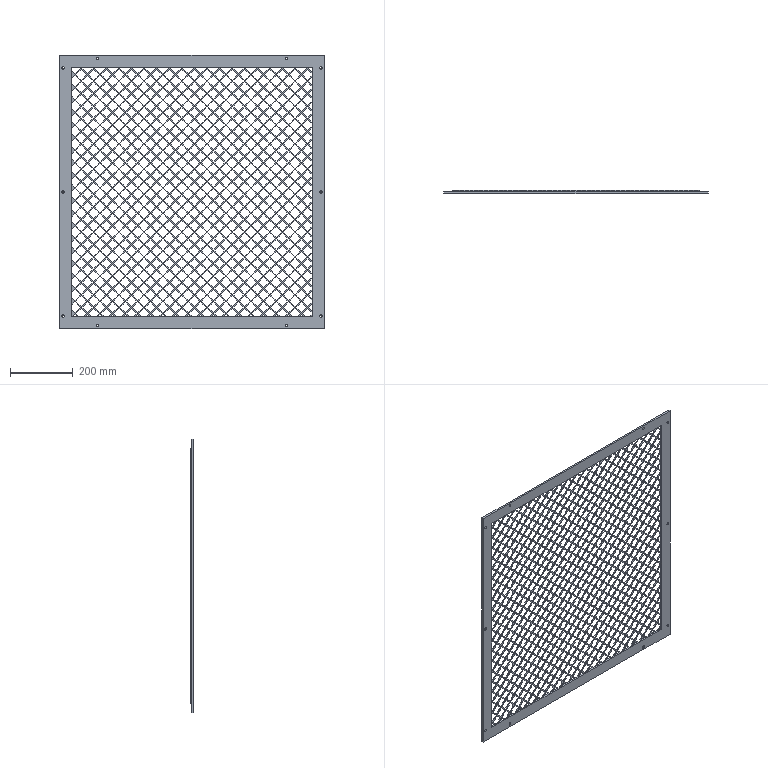Part | STEP file | OP10-005_side cover | 3 solids | 3447 faces | volume 1174721 mm3 | plane 3427 | cylinder 20 | commonest cylinder face diameters 8 x20